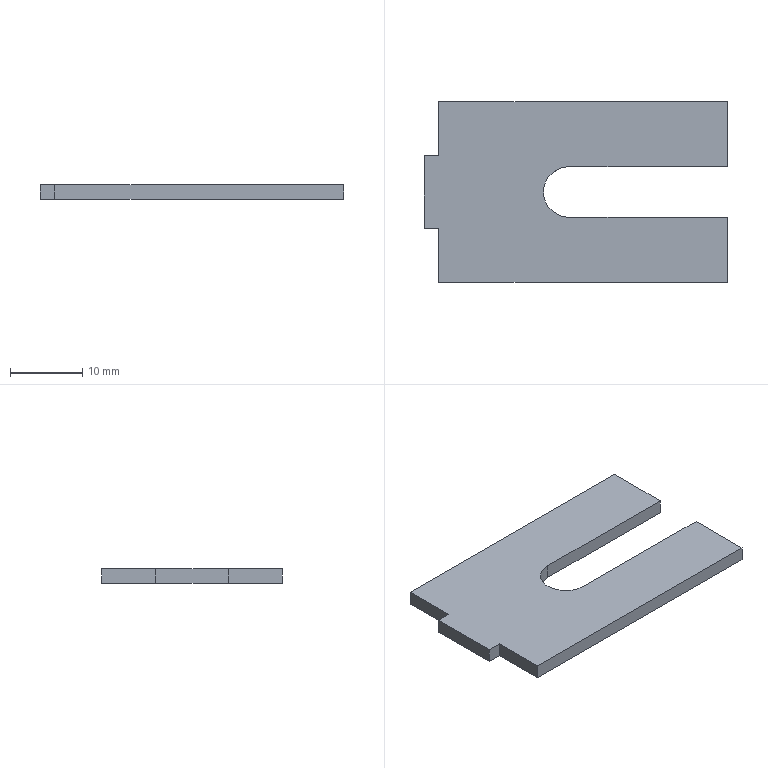Part | STEP file | xzz-001-1-01 | 1 solid | 14 faces | box 42 x 25 x 2 mm | volume 1694 mm3 | plane 13 | cylinder 1 | commonest cylinder face diameters 7 x1
STEP:
#1=CARTESIAN_POINT('',(143.416,-26.648,-2.));
#2=VERTEX_POINT('',#1);
#3=CARTESIAN_POINT('',(103.416,-26.648,-2.));
#4=VERTEX_POINT('',#3);
#5=CARTESIAN_POINT('',(121.416,-26.648,-2.));
#6=DIRECTION('',(-1.,0.,0.));
#7=VECTOR('',#6,1000.);
#8=LINE('',#5,#7);
#9=EDGE_CURVE('',#2,#4,#8,.T.);
#10=ORIENTED_EDGE('',*,*,#9,.F.);
#11=CARTESIAN_POINT('',(143.416,-35.648,-2.));
#12=VERTEX_POINT('',#11);
#13=CARTESIAN_POINT('',(143.416,-39.148,-2.));
#14=DIRECTION('',(0.,1.,0.));
#15=VECTOR('',#14,1000.);
#16=LINE('',#13,#15);
#17=EDGE_CURVE('',#12,#2,#16,.T.);
#18=ORIENTED_EDGE('',*,*,#17,.F.);
#19=CARTESIAN_POINT('',(121.416,-35.648,-2.));
#20=VERTEX_POINT('',#19);
#21=CARTESIAN_POINT('',(121.416,-35.648,-2.));
#22=DIRECTION('',(1.,0.,0.));
#23=VECTOR('',#22,1000.);
#24=LINE('',#21,#23);
#25=EDGE_CURVE('',#20,#12,#24,.T.);
#26=ORIENTED_EDGE('',*,*,#25,.F.);
#27=CARTESIAN_POINT('',(121.416,-42.648,-2.));
#28=VERTEX_POINT('',#27);
#29=CARTESIAN_POINT('',(121.416,-39.148,-2.));
#30=DIRECTION('',(0.,0.,-1.));
#31=DIRECTION('',(1.,0.,0.));
#32=AXIS2_PLACEMENT_3D('',#29,#30,#31);
#33=CIRCLE('',#32,3.5);
#34=EDGE_CURVE('',#28,#20,#33,.T.);
#35=ORIENTED_EDGE('',*,*,#34,.F.);
#36=CARTESIAN_POINT('',(143.416,-42.648,-2.));
#37=VERTEX_POINT('',#36);
#38=CARTESIAN_POINT('',(121.416,-42.648,-2.));
#39=DIRECTION('',(-1.,0.,0.));
#40=VECTOR('',#39,1000.);
#41=LINE('',#38,#40);
#42=EDGE_CURVE('',#37,#28,#41,.T.);
#43=ORIENTED_EDGE('',*,*,#42,.F.);
#44=CARTESIAN_POINT('',(143.416,-51.648,-2.));
#45=VERTEX_POINT('',#44);
#46=CARTESIAN_POINT('',(143.416,-39.148,-2.));
#47=DIRECTION('',(0.,1.,0.));
#48=VECTOR('',#47,1000.);
#49=LINE('',#46,#48);
#50=EDGE_CURVE('',#45,#37,#49,.T.);
#51=ORIENTED_EDGE('',*,*,#50,.F.);
#52=CARTESIAN_POINT('',(103.416,-51.648,-2.));
#53=VERTEX_POINT('',#52);
#54=CARTESIAN_POINT('',(121.416,-51.648,-2.));
#55=DIRECTION('',(1.,0.,0.));
#56=VECTOR('',#55,1000.);
#57=LINE('',#54,#56);
#58=EDGE_CURVE('',#53,#45,#57,.T.);
#59=ORIENTED_EDGE('',*,*,#58,.F.);
#60=CARTESIAN_POINT('',(103.416,-44.148,-2.));
#61=VERTEX_POINT('',#60);
#62=CARTESIAN_POINT('',(103.416,-39.148,-2.));
#63=DIRECTION('',(0.,-1.,0.));
#64=VECTOR('',#63,1000.);
#65=LINE('',#62,#64);
#66=EDGE_CURVE('',#61,#53,#65,.T.);
#67=ORIENTED_EDGE('',*,*,#66,.F.);
#68=CARTESIAN_POINT('',(101.416,-44.148,-2.));
#69=VERTEX_POINT('',#68);
#70=CARTESIAN_POINT('',(121.416,-44.148,-2.));
#71=DIRECTION('',(1.,0.,0.));
#72=VECTOR('',#71,1000.);
#73=LINE('',#70,#72);
#74=EDGE_CURVE('',#69,#61,#73,.T.);
#75=ORIENTED_EDGE('',*,*,#74,.F.);
#76=CARTESIAN_POINT('',(101.416,-34.148,-2.));
#77=VERTEX_POINT('',#76);
#78=CARTESIAN_POINT('',(101.416,-39.148,-2.));
#79=DIRECTION('',(0.,-1.,0.));
#80=VECTOR('',#79,1000.);
#81=LINE('',#78,#80);
#82=EDGE_CURVE('',#77,#69,#81,.T.);
#83=ORIENTED_EDGE('',*,*,#82,.F.);
#84=CARTESIAN_POINT('',(103.416,-34.148,-2.));
#85=VERTEX_POINT('',#84);
#86=CARTESIAN_POINT('',(121.416,-34.148,-2.));
#87=DIRECTION('',(-1.,0.,0.));
#88=VECTOR('',#87,1000.);
#89=LINE('',#86,#88);
#90=EDGE_CURVE('',#85,#77,#89,.T.);
#91=ORIENTED_EDGE('',*,*,#90,.F.);
#92=CARTESIAN_POINT('',(103.416,-39.148,-2.));
#93=DIRECTION('',(0.,-1.,0.));
#94=VECTOR('',#93,1000.);
#95=LINE('',#92,#94);
#96=EDGE_CURVE('',#4,#85,#95,.T.);
#97=ORIENTED_EDGE('',*,*,#96,.F.);
#98=EDGE_LOOP('',(#10,#18,#26,#35,#43,#51,#59,#67,#75,#83,#91,#97));
#99=FACE_OUTER_BOUND('',#98,.T.);
#100=CARTESIAN_POINT('',(121.416,-39.148,-2.));
#101=DIRECTION('',(0.,0.,1.));
#102=DIRECTION('',(1.,0.,0.));
#103=AXIS2_PLACEMENT_3D('',#100,#101,#102);
#104=PLANE('',#103);
#105=ADVANCED_FACE('',(#99),#104,.F.);
#106=ORIENTED_EDGE('',*,*,#96,.T.);
#107=CARTESIAN_POINT('',(103.416,-34.148,0.));
#108=VERTEX_POINT('',#107);
#109=CARTESIAN_POINT('',(103.416,-34.148,-2.));
#110=DIRECTION('',(0.,0.,1.));
#111=VECTOR('',#110,1000.);
#112=LINE('',#109,#111);
#113=EDGE_CURVE('',#85,#108,#112,.T.);
#114=ORIENTED_EDGE('',*,*,#113,.T.);
#115=CARTESIAN_POINT('',(103.416,-26.648,0.));
#116=VERTEX_POINT('',#115);
#117=CARTESIAN_POINT('',(103.416,-26.648,0.));
#118=DIRECTION('',(0.,1.,0.));
#119=VECTOR('',#118,1000.);
#120=LINE('',#117,#119);
#121=EDGE_CURVE('',#108,#116,#120,.T.);
#122=ORIENTED_EDGE('',*,*,#121,.T.);
#123=CARTESIAN_POINT('',(103.416,-26.648,-2.));
#124=DIRECTION('',(0.,0.,-1.));
#125=VECTOR('',#124,1000.);
#126=LINE('',#123,#125);
#127=EDGE_CURVE('',#116,#4,#126,.T.);
#128=ORIENTED_EDGE('',*,*,#127,.T.);
#129=EDGE_LOOP('',(#106,#114,#122,#128));
#130=FACE_OUTER_BOUND('',#129,.T.);
#131=CARTESIAN_POINT('',(103.416,-26.648,-2.));
#132=DIRECTION('',(-1.,0.,0.));
#133=DIRECTION('',(0.,0.,1.));
#134=AXIS2_PLACEMENT_3D('',#131,#132,#133);
#135=PLANE('',#134);
#136=ADVANCED_FACE('',(#130),#135,.T.);
#137=ORIENTED_EDGE('',*,*,#9,.T.);
#138=ORIENTED_EDGE('',*,*,#127,.F.);
#139=CARTESIAN_POINT('',(143.416,-26.648,0.));
#140=VERTEX_POINT('',#139);
#141=CARTESIAN_POINT('',(103.416,-26.648,0.));
#142=DIRECTION('',(1.,0.,0.));
#143=VECTOR('',#142,1000.);
#144=LINE('',#141,#143);
#145=EDGE_CURVE('',#116,#140,#144,.T.);
#146=ORIENTED_EDGE('',*,*,#145,.T.);
#147=CARTESIAN_POINT('',(143.416,-26.648,-2.));
#148=DIRECTION('',(0.,0.,-1.));
#149=VECTOR('',#148,1000.);
#150=LINE('',#147,#149);
#151=EDGE_CURVE('',#140,#2,#150,.T.);
#152=ORIENTED_EDGE('',*,*,#151,.T.);
#153=EDGE_LOOP('',(#137,#138,#146,#152));
#154=FACE_OUTER_BOUND('',#153,.T.);
#155=CARTESIAN_POINT('',(103.416,-26.648,-2.));
#156=DIRECTION('',(0.,1.,0.));
#157=DIRECTION('',(0.,0.,1.));
#158=AXIS2_PLACEMENT_3D('',#155,#156,#157);
#159=PLANE('',#158);
#160=ADVANCED_FACE('',(#154),#159,.T.);
#161=ORIENTED_EDGE('',*,*,#17,.T.);
#162=ORIENTED_EDGE('',*,*,#151,.F.);
#163=CARTESIAN_POINT('',(143.416,-35.648,0.));
#164=VERTEX_POINT('',#163);
#165=CARTESIAN_POINT('',(143.416,-26.648,0.));
#166=DIRECTION('',(0.,-1.,0.));
#167=VECTOR('',#166,1000.);
#168=LINE('',#165,#167);
#169=EDGE_CURVE('',#140,#164,#168,.T.);
#170=ORIENTED_EDGE('',*,*,#169,.T.);
#171=CARTESIAN_POINT('',(143.416,-35.648,-2.));
#172=DIRECTION('',(0.,0.,-1.));
#173=VECTOR('',#172,1000.);
#174=LINE('',#171,#173);
#175=EDGE_CURVE('',#164,#12,#174,.T.);
#176=ORIENTED_EDGE('',*,*,#175,.T.);
#177=EDGE_LOOP('',(#161,#162,#170,#176));
#178=FACE_OUTER_BOUND('',#177,.T.);
#179=CARTESIAN_POINT('',(143.416,-26.648,-2.));
#180=DIRECTION('',(1.,0.,0.));
#181=DIRECTION('',(0.,0.,-1.));
#182=AXIS2_PLACEMENT_3D('',#179,#180,#181);
#183=PLANE('',#182);
#184=ADVANCED_FACE('',(#178),#183,.T.);
#185=ORIENTED_EDGE('',*,*,#25,.T.);
#186=ORIENTED_EDGE('',*,*,#175,.F.);
#187=CARTESIAN_POINT('',(121.416,-35.648,0.));
#188=VERTEX_POINT('',#187);
#189=CARTESIAN_POINT('',(121.416,-35.648,0.));
#190=DIRECTION('',(-1.,0.,0.));
#191=VECTOR('',#190,1000.);
#192=LINE('',#189,#191);
#193=EDGE_CURVE('',#164,#188,#192,.T.);
#194=ORIENTED_EDGE('',*,*,#193,.T.);
#195=CARTESIAN_POINT('',(121.416,-35.648,-2.));
#196=DIRECTION('',(0.,0.,-1.));
#197=VECTOR('',#196,1000.);
#198=LINE('',#195,#197);
#199=EDGE_CURVE('',#188,#20,#198,.T.);
#200=ORIENTED_EDGE('',*,*,#199,.T.);
#201=EDGE_LOOP('',(#185,#186,#194,#200));
#202=FACE_OUTER_BOUND('',#201,.T.);
#203=CARTESIAN_POINT('',(121.416,-35.648,-2.));
#204=DIRECTION('',(0.,-1.,0.));
#205=DIRECTION('',(1.,0.,0.));
#206=AXIS2_PLACEMENT_3D('',#203,#204,#205);
#207=PLANE('',#206);
#208=ADVANCED_FACE('',(#202),#207,.T.);
#209=CARTESIAN_POINT('',(121.416,-42.648,0.));
#210=VERTEX_POINT('',#209);
#211=CARTESIAN_POINT('',(121.416,-42.648,-2.));
#212=DIRECTION('',(0.,0.,1.));
#213=VECTOR('',#212,1000.);
#214=LINE('',#211,#213);
#215=EDGE_CURVE('',#28,#210,#214,.T.);
#216=ORIENTED_EDGE('',*,*,#215,.F.);
#217=ORIENTED_EDGE('',*,*,#34,.T.);
#218=ORIENTED_EDGE('',*,*,#199,.F.);
#219=CARTESIAN_POINT('',(121.416,-39.148,0.));
#220=DIRECTION('',(0.,0.,-1.));
#221=DIRECTION('',(1.,0.,0.));
#222=AXIS2_PLACEMENT_3D('',#219,#220,#221);
#223=CIRCLE('',#222,3.5);
#224=EDGE_CURVE('',#210,#188,#223,.T.);
#225=ORIENTED_EDGE('',*,*,#224,.F.);
#226=EDGE_LOOP('',(#216,#217,#218,#225));
#227=FACE_OUTER_BOUND('',#226,.T.);
#228=CARTESIAN_POINT('',(121.416,-39.148,-2.));
#229=DIRECTION('',(0.,0.,1.));
#230=DIRECTION('',(1.,0.,0.));
#231=AXIS2_PLACEMENT_3D('',#228,#229,#230);
#232=CYLINDRICAL_SURFACE('',#231,3.5);
#233=ADVANCED_FACE('',(#227),#232,.F.);
#234=ORIENTED_EDGE('',*,*,#42,.T.);
#235=ORIENTED_EDGE('',*,*,#215,.T.);
#236=CARTESIAN_POINT('',(143.416,-42.648,0.));
#237=VERTEX_POINT('',#236);
#238=CARTESIAN_POINT('',(121.416,-42.648,0.));
#239=DIRECTION('',(1.,0.,0.));
#240=VECTOR('',#239,1000.);
#241=LINE('',#238,#240);
#242=EDGE_CURVE('',#210,#237,#241,.T.);
#243=ORIENTED_EDGE('',*,*,#242,.T.);
#244=CARTESIAN_POINT('',(143.416,-42.648,-2.));
#245=DIRECTION('',(0.,0.,-1.));
#246=VECTOR('',#245,1000.);
#247=LINE('',#244,#246);
#248=EDGE_CURVE('',#237,#37,#247,.T.);
#249=ORIENTED_EDGE('',*,*,#248,.T.);
#250=EDGE_LOOP('',(#234,#235,#243,#249));
#251=FACE_OUTER_BOUND('',#250,.T.);
#252=CARTESIAN_POINT('',(121.416,-42.648,-2.));
#253=DIRECTION('',(0.,1.,0.));
#254=DIRECTION('',(0.,0.,1.));
#255=AXIS2_PLACEMENT_3D('',#252,#253,#254);
#256=PLANE('',#255);
#257=ADVANCED_FACE('',(#251),#256,.T.);
#258=ORIENTED_EDGE('',*,*,#50,.T.);
#259=ORIENTED_EDGE('',*,*,#248,.F.);
#260=CARTESIAN_POINT('',(143.416,-51.648,0.));
#261=VERTEX_POINT('',#260);
#262=CARTESIAN_POINT('',(143.416,-42.648,0.));
#263=DIRECTION('',(0.,-1.,0.));
#264=VECTOR('',#263,1000.);
#265=LINE('',#262,#264);
#266=EDGE_CURVE('',#237,#261,#265,.T.);
#267=ORIENTED_EDGE('',*,*,#266,.T.);
#268=CARTESIAN_POINT('',(143.416,-51.648,-2.));
#269=DIRECTION('',(0.,0.,-1.));
#270=VECTOR('',#269,1000.);
#271=LINE('',#268,#270);
#272=EDGE_CURVE('',#261,#45,#271,.T.);
#273=ORIENTED_EDGE('',*,*,#272,.T.);
#274=EDGE_LOOP('',(#258,#259,#267,#273));
#275=FACE_OUTER_BOUND('',#274,.T.);
#276=CARTESIAN_POINT('',(143.416,-42.648,-2.));
#277=DIRECTION('',(1.,0.,0.));
#278=DIRECTION('',(0.,0.,-1.));
#279=AXIS2_PLACEMENT_3D('',#276,#277,#278);
#280=PLANE('',#279);
#281=ADVANCED_FACE('',(#275),#280,.T.);
#282=ORIENTED_EDGE('',*,*,#58,.T.);
#283=ORIENTED_EDGE('',*,*,#272,.F.);
#284=CARTESIAN_POINT('',(103.416,-51.648,0.));
#285=VERTEX_POINT('',#284);
#286=CARTESIAN_POINT('',(103.416,-51.648,0.));
#287=DIRECTION('',(-1.,0.,0.));
#288=VECTOR('',#287,1000.);
#289=LINE('',#286,#288);
#290=EDGE_CURVE('',#261,#285,#289,.T.);
#291=ORIENTED_EDGE('',*,*,#290,.T.);
#292=CARTESIAN_POINT('',(103.416,-51.648,-2.));
#293=DIRECTION('',(0.,0.,-1.));
#294=VECTOR('',#293,1000.);
#295=LINE('',#292,#294);
#296=EDGE_CURVE('',#285,#53,#295,.T.);
#297=ORIENTED_EDGE('',*,*,#296,.T.);
#298=EDGE_LOOP('',(#282,#283,#291,#297));
#299=FACE_OUTER_BOUND('',#298,.T.);
#300=CARTESIAN_POINT('',(103.416,-51.648,-2.));
#301=DIRECTION('',(0.,-1.,0.));
#302=DIRECTION('',(0.,0.,-1.));
#303=AXIS2_PLACEMENT_3D('',#300,#301,#302);
#304=PLANE('',#303);
#305=ADVANCED_FACE('',(#299),#304,.T.);
#306=ORIENTED_EDGE('',*,*,#66,.T.);
#307=ORIENTED_EDGE('',*,*,#296,.F.);
#308=CARTESIAN_POINT('',(103.416,-44.148,0.));
#309=VERTEX_POINT('',#308);
#310=CARTESIAN_POINT('',(103.416,-44.148,0.));
#311=DIRECTION('',(0.,1.,0.));
#312=VECTOR('',#311,1000.);
#313=LINE('',#310,#312);
#314=EDGE_CURVE('',#285,#309,#313,.T.);
#315=ORIENTED_EDGE('',*,*,#314,.T.);
#316=CARTESIAN_POINT('',(103.416,-44.148,-2.));
#317=DIRECTION('',(0.,0.,-1.));
#318=VECTOR('',#317,1000.);
#319=LINE('',#316,#318);
#320=EDGE_CURVE('',#309,#61,#319,.T.);
#321=ORIENTED_EDGE('',*,*,#320,.T.);
#322=EDGE_LOOP('',(#306,#307,#315,#321));
#323=FACE_OUTER_BOUND('',#322,.T.);
#324=CARTESIAN_POINT('',(103.416,-44.148,-2.));
#325=DIRECTION('',(-1.,0.,0.));
#326=DIRECTION('',(0.,0.,1.));
#327=AXIS2_PLACEMENT_3D('',#324,#325,#326);
#328=PLANE('',#327);
#329=ADVANCED_FACE('',(#323),#328,.T.);
#330=ORIENTED_EDGE('',*,*,#74,.T.);
#331=ORIENTED_EDGE('',*,*,#320,.F.);
#332=CARTESIAN_POINT('',(101.416,-44.148,0.));
#333=VERTEX_POINT('',#332);
#334=CARTESIAN_POINT('',(103.416,-44.148,0.));
#335=DIRECTION('',(-1.,0.,0.));
#336=VECTOR('',#335,1000.);
#337=LINE('',#334,#336);
#338=EDGE_CURVE('',#309,#333,#337,.T.);
#339=ORIENTED_EDGE('',*,*,#338,.T.);
#340=CARTESIAN_POINT('',(101.416,-44.148,-2.));
#341=DIRECTION('',(0.,0.,-1.));
#342=VECTOR('',#341,1000.);
#343=LINE('',#340,#342);
#344=EDGE_CURVE('',#333,#69,#343,.T.);
#345=ORIENTED_EDGE('',*,*,#344,.T.);
#346=EDGE_LOOP('',(#330,#331,#339,#345));
#347=FACE_OUTER_BOUND('',#346,.T.);
#348=CARTESIAN_POINT('',(103.416,-44.148,-2.));
#349=DIRECTION('',(0.,-1.,0.));
#350=DIRECTION('',(0.,0.,-1.));
#351=AXIS2_PLACEMENT_3D('',#348,#349,#350);
#352=PLANE('',#351);
#353=ADVANCED_FACE('',(#347),#352,.T.);
#354=ORIENTED_EDGE('',*,*,#82,.T.);
#355=ORIENTED_EDGE('',*,*,#344,.F.);
#356=CARTESIAN_POINT('',(101.416,-34.148,0.));
#357=VERTEX_POINT('',#356);
#358=CARTESIAN_POINT('',(101.416,-34.148,0.));
#359=DIRECTION('',(0.,1.,0.));
#360=VECTOR('',#359,1000.);
#361=LINE('',#358,#360);
#362=EDGE_CURVE('',#333,#357,#361,.T.);
#363=ORIENTED_EDGE('',*,*,#362,.T.);
#364=CARTESIAN_POINT('',(101.416,-34.148,-2.));
#365=DIRECTION('',(0.,0.,-1.));
#366=VECTOR('',#365,1000.);
#367=LINE('',#364,#366);
#368=EDGE_CURVE('',#357,#77,#367,.T.);
#369=ORIENTED_EDGE('',*,*,#368,.T.);
#370=EDGE_LOOP('',(#354,#355,#363,#369));
#371=FACE_OUTER_BOUND('',#370,.T.);
#372=CARTESIAN_POINT('',(101.416,-34.148,-2.));
#373=DIRECTION('',(-1.,0.,0.));
#374=DIRECTION('',(0.,0.,1.));
#375=AXIS2_PLACEMENT_3D('',#372,#373,#374);
#376=PLANE('',#375);
#377=ADVANCED_FACE('',(#371),#376,.T.);
#378=ORIENTED_EDGE('',*,*,#90,.T.);
#379=ORIENTED_EDGE('',*,*,#368,.F.);
#380=CARTESIAN_POINT('',(103.416,-34.148,0.));
#381=DIRECTION('',(1.,0.,0.));
#382=VECTOR('',#381,1000.);
#383=LINE('',#380,#382);
#384=EDGE_CURVE('',#357,#108,#383,.T.);
#385=ORIENTED_EDGE('',*,*,#384,.T.);
#386=ORIENTED_EDGE('',*,*,#113,.F.);
#387=EDGE_LOOP('',(#378,#379,#385,#386));
#388=FACE_OUTER_BOUND('',#387,.T.);
#389=CARTESIAN_POINT('',(103.416,-34.148,-2.));
#390=DIRECTION('',(0.,1.,0.));
#391=DIRECTION('',(-1.,0.,0.));
#392=AXIS2_PLACEMENT_3D('',#389,#390,#391);
#393=PLANE('',#392);
#394=ADVANCED_FACE('',(#388),#393,.T.);
#395=ORIENTED_EDGE('',*,*,#169,.F.);
#396=ORIENTED_EDGE('',*,*,#145,.F.);
#397=ORIENTED_EDGE('',*,*,#121,.F.);
#398=ORIENTED_EDGE('',*,*,#384,.F.);
#399=ORIENTED_EDGE('',*,*,#362,.F.);
#400=ORIENTED_EDGE('',*,*,#338,.F.);
#401=ORIENTED_EDGE('',*,*,#314,.F.);
#402=ORIENTED_EDGE('',*,*,#290,.F.);
#403=ORIENTED_EDGE('',*,*,#266,.F.);
#404=ORIENTED_EDGE('',*,*,#242,.F.);
#405=ORIENTED_EDGE('',*,*,#224,.T.);
#406=ORIENTED_EDGE('',*,*,#193,.F.);
#407=EDGE_LOOP('',(#395,#396,#397,#398,#399,#400,#401,#402,#403,#404,#405,#406));
#408=FACE_OUTER_BOUND('',#407,.T.);
#409=CARTESIAN_POINT('',(121.416,-39.148,0.));
#410=DIRECTION('',(0.,0.,1.));
#411=DIRECTION('',(1.,0.,0.));
#412=AXIS2_PLACEMENT_3D('',#409,#410,#411);
#413=PLANE('',#412);
#414=ADVANCED_FACE('',(#408),#413,.T.);
#415=CLOSED_SHELL('',(#105,#136,#160,#184,#208,#233,#257,#281,#305,#329,#353,#377,#394,#414));
#416=MANIFOLD_SOLID_BREP('',#415);
#417=CARTESIAN_POINT('',(0.,0.,0.));
#418=DIRECTION('',(0.,0.,1.));
#419=DIRECTION('',(1.,0.,0.));
#420=AXIS2_PLACEMENT_3D('',#417,#418,#419);
#421=(LENGTH_UNIT()NAMED_UNIT(*)SI_UNIT(.MILLI.,.METRE.));
#422=UNCERTAINTY_MEASURE_WITH_UNIT(LENGTH_MEASURE(0.00001),#421,'','');
#423=(NAMED_UNIT(*)PLANE_ANGLE_UNIT()SI_UNIT($,.RADIAN.));
#424=(NAMED_UNIT(*)SI_UNIT($,.STERADIAN.)SOLID_ANGLE_UNIT());
#425=(GEOMETRIC_REPRESENTATION_CONTEXT(3)GLOBAL_UNCERTAINTY_ASSIGNED_CONTEXT((#422))GLOBAL_UNIT_ASSIGNED_CONTEXT((#421,#423,#424))REPRESENTATION_CONTEXT('',''));
#426=ADVANCED_BREP_SHAPE_REPRESENTATION('',(#416,#420),#425);